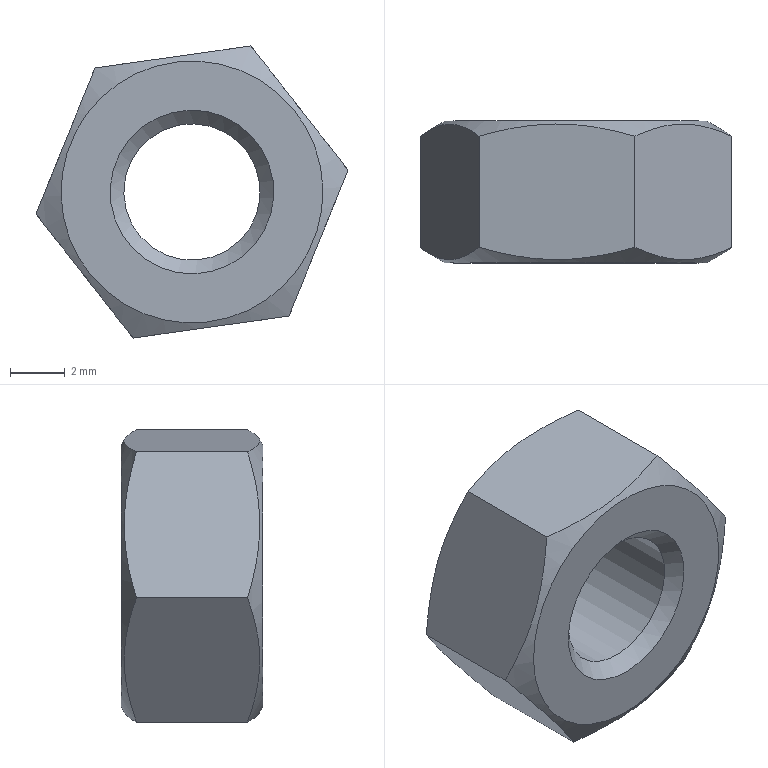Part | NX | features 倒角1 2 | 1 solid | 13 faces | box 11.434 x 5.2 x 10.707 mm | volume 339.24 mm3 | plane 8 | cone 4 | cylinder 1 | commonest cylinder face diameters 5 x1
STEP:
#1=CARTESIAN_POINT('',(16.564,347.416,103.063));
#2=VERTEX_POINT('',#1);
#3=CARTESIAN_POINT('',(17.5,347.416,105.381));
#4=DIRECTION('',(0.,1.,0.));
#5=DIRECTION('',(-0.3744,0.,-0.9273));
#6=AXIS2_PLACEMENT_3D('',#3,#4,#5);
#7=CIRCLE('',#6,2.5);
#8=EDGE_CURVE('',#2,#2,#7,.T.);
#9=ORIENTED_EDGE('',*,*,#8,.F.);
#10=EDGE_LOOP('',(#9));
#11=FACE_BOUND('',#10,.T.);
#12=CARTESIAN_POINT('',(16.377,347.916,102.599));
#13=VERTEX_POINT('',#12);
#14=CARTESIAN_POINT('',(17.5,347.916,105.381));
#15=DIRECTION('',(0.,-1.,0.));
#16=DIRECTION('',(-0.3744,0.,-0.9273));
#17=AXIS2_PLACEMENT_3D('',#14,#15,#16);
#18=CIRCLE('',#17,3.);
#19=EDGE_CURVE('',#13,#13,#18,.T.);
#20=ORIENTED_EDGE('',*,*,#19,.F.);
#21=EDGE_LOOP('',(#20));
#22=FACE_BOUND('',#21,.T.);
#23=CARTESIAN_POINT('',(17.5,347.416,105.381));
#24=DIRECTION('',(0.,1.,0.));
#25=DIRECTION('',(0.3744,0.,0.9273));
#26=AXIS2_PLACEMENT_3D('',#23,#24,#25);
#27=CONICAL_SURFACE('',#26,2.5,0.7854);
#28=ADVANCED_FACE('',(#11,#22),#27,.F.);
#29=CARTESIAN_POINT('',(16.377,342.716,102.599));
#30=VERTEX_POINT('',#29);
#31=CARTESIAN_POINT('',(17.5,342.716,105.381));
#32=DIRECTION('',(0.,1.,0.));
#33=DIRECTION('',(-0.3744,0.,-0.9273));
#34=AXIS2_PLACEMENT_3D('',#31,#32,#33);
#35=CIRCLE('',#34,3.);
#36=EDGE_CURVE('',#30,#30,#35,.T.);
#37=ORIENTED_EDGE('',*,*,#36,.F.);
#38=EDGE_LOOP('',(#37));
#39=FACE_BOUND('',#38,.T.);
#40=CARTESIAN_POINT('',(16.564,343.216,103.063));
#41=VERTEX_POINT('',#40);
#42=CARTESIAN_POINT('',(17.5,343.216,105.381));
#43=DIRECTION('',(0.,-1.,0.));
#44=DIRECTION('',(-0.3744,0.,-0.9273));
#45=AXIS2_PLACEMENT_3D('',#42,#43,#44);
#46=CIRCLE('',#45,2.5);
#47=EDGE_CURVE('',#41,#41,#46,.T.);
#48=ORIENTED_EDGE('',*,*,#47,.F.);
#49=EDGE_LOOP('',(#48));
#50=FACE_BOUND('',#49,.T.);
#51=CARTESIAN_POINT('',(17.5,342.716,105.381));
#52=DIRECTION('',(0.,-1.,0.));
#53=DIRECTION('',(-0.3744,0.,-0.9273));
#54=AXIS2_PLACEMENT_3D('',#51,#52,#53);
#55=CONICAL_SURFACE('',#54,3.,0.7854);
#56=ADVANCED_FACE('',(#39,#50),#55,.F.);
#57=CARTESIAN_POINT('',(13.945,347.354,109.93));
#58=VERTEX_POINT('',#57);
#59=CARTESIAN_POINT('',(19.662,347.354,110.735));
#60=VERTEX_POINT('',#59);
#61=CARTESIAN_POINT('',(13.945,347.354,109.93));
#62=CARTESIAN_POINT('',(14.878,347.626,110.061));
#63=CARTESIAN_POINT('',(16.793,347.975,110.331));
#64=CARTESIAN_POINT('',(18.727,347.626,110.603));
#65=CARTESIAN_POINT('',(19.662,347.354,110.735));
#66=B_SPLINE_CURVE_WITH_KNOTS('',3,(#61,#62,#63,#64,#65),.UNSPECIFIED.,.F.,.F.,(4,1,4),(0.,0.002915,0.005831),.UNSPECIFIED.);
#67=EDGE_CURVE('',#58,#60,#66,.T.);
#68=ORIENTED_EDGE('',*,*,#67,.T.);
#69=CARTESIAN_POINT('',(23.217,347.354,106.186));
#70=VERTEX_POINT('',#69);
#71=CARTESIAN_POINT('',(19.662,347.354,110.735));
#72=CARTESIAN_POINT('',(20.242,347.626,109.992));
#73=CARTESIAN_POINT('',(21.433,347.975,108.469));
#74=CARTESIAN_POINT('',(22.636,347.626,106.93));
#75=CARTESIAN_POINT('',(23.217,347.354,106.186));
#76=B_SPLINE_CURVE_WITH_KNOTS('',3,(#71,#72,#73,#74,#75),.UNSPECIFIED.,.F.,.F.,(4,1,4),(0.,0.002915,0.005831),.UNSPECIFIED.);
#77=EDGE_CURVE('',#60,#70,#76,.T.);
#78=ORIENTED_EDGE('',*,*,#77,.T.);
#79=CARTESIAN_POINT('',(21.055,347.354,100.832));
#80=VERTEX_POINT('',#79);
#81=CARTESIAN_POINT('',(23.217,347.354,106.186));
#82=CARTESIAN_POINT('',(22.864,347.626,105.312));
#83=CARTESIAN_POINT('',(22.14,347.975,103.519));
#84=CARTESIAN_POINT('',(21.409,347.626,101.708));
#85=CARTESIAN_POINT('',(21.055,347.354,100.832));
#86=B_SPLINE_CURVE_WITH_KNOTS('',3,(#81,#82,#83,#84,#85),.UNSPECIFIED.,.F.,.F.,(4,1,4),(0.,0.002915,0.005831),.UNSPECIFIED.);
#87=EDGE_CURVE('',#70,#80,#86,.T.);
#88=ORIENTED_EDGE('',*,*,#87,.T.);
#89=CARTESIAN_POINT('',(15.338,347.354,100.028));
#90=VERTEX_POINT('',#89);
#91=CARTESIAN_POINT('',(21.055,347.354,100.832));
#92=CARTESIAN_POINT('',(20.122,347.626,100.701));
#93=CARTESIAN_POINT('',(18.207,347.975,100.431));
#94=CARTESIAN_POINT('',(16.273,347.626,100.159));
#95=CARTESIAN_POINT('',(15.338,347.354,100.028));
#96=B_SPLINE_CURVE_WITH_KNOTS('',3,(#91,#92,#93,#94,#95),.UNSPECIFIED.,.F.,.F.,(4,1,4),(0.,0.002915,0.005831),.UNSPECIFIED.);
#97=EDGE_CURVE('',#80,#90,#96,.T.);
#98=ORIENTED_EDGE('',*,*,#97,.T.);
#99=CARTESIAN_POINT('',(11.783,347.354,104.576));
#100=VERTEX_POINT('',#99);
#101=CARTESIAN_POINT('',(15.338,347.354,100.028));
#102=CARTESIAN_POINT('',(14.758,347.626,100.77));
#103=CARTESIAN_POINT('',(13.567,347.975,102.294));
#104=CARTESIAN_POINT('',(12.364,347.626,103.833));
#105=CARTESIAN_POINT('',(11.783,347.354,104.576));
#106=B_SPLINE_CURVE_WITH_KNOTS('',3,(#101,#102,#103,#104,#105),.UNSPECIFIED.,.F.,.F.,(4,1,4),(0.,0.002915,0.005831),.UNSPECIFIED.);
#107=EDGE_CURVE('',#90,#100,#106,.T.);
#108=ORIENTED_EDGE('',*,*,#107,.T.);
#109=CARTESIAN_POINT('',(11.783,347.354,104.576));
#110=CARTESIAN_POINT('',(12.136,347.626,105.451));
#111=CARTESIAN_POINT('',(12.86,347.975,107.244));
#112=CARTESIAN_POINT('',(13.591,347.626,109.055));
#113=CARTESIAN_POINT('',(13.945,347.354,109.93));
#114=B_SPLINE_CURVE_WITH_KNOTS('',3,(#109,#110,#111,#112,#113),.UNSPECIFIED.,.F.,.F.,(4,1,4),(0.,0.002915,0.005831),.UNSPECIFIED.);
#115=EDGE_CURVE('',#100,#58,#114,.T.);
#116=ORIENTED_EDGE('',*,*,#115,.T.);
#117=EDGE_LOOP('',(#68,#78,#88,#98,#108,#116));
#118=FACE_BOUND('',#117,.T.);
#119=CARTESIAN_POINT('',(19.297,347.916,109.832));
#120=VERTEX_POINT('',#119);
#121=CARTESIAN_POINT('',(17.5,347.916,105.381));
#122=DIRECTION('',(0.,-1.,0.));
#123=DIRECTION('',(0.3744,0.,0.9273));
#124=AXIS2_PLACEMENT_3D('',#121,#122,#123);
#125=CIRCLE('',#124,4.8);
#126=EDGE_CURVE('',#120,#120,#125,.T.);
#127=ORIENTED_EDGE('',*,*,#126,.T.);
#128=EDGE_LOOP('',(#127));
#129=FACE_BOUND('',#128,.T.);
#130=CARTESIAN_POINT('',(17.5,347.354,105.381));
#131=DIRECTION('',(0.,-1.,0.));
#132=DIRECTION('',(-0.3744,0.,-0.9273));
#133=AXIS2_PLACEMENT_3D('',#130,#131,#132);
#134=CONICAL_SURFACE('',#133,5.774,1.047);
#135=ADVANCED_FACE('',(#118,#129),#134,.T.);
#136=CARTESIAN_POINT('',(19.297,342.716,109.832));
#137=VERTEX_POINT('',#136);
#138=CARTESIAN_POINT('',(17.5,342.716,105.381));
#139=DIRECTION('',(0.,-1.,0.));
#140=DIRECTION('',(0.3744,0.,0.9273));
#141=AXIS2_PLACEMENT_3D('',#138,#139,#140);
#142=CIRCLE('',#141,4.8);
#143=EDGE_CURVE('',#137,#137,#142,.T.);
#144=ORIENTED_EDGE('',*,*,#143,.F.);
#145=EDGE_LOOP('',(#144));
#146=FACE_BOUND('',#145,.T.);
#147=CARTESIAN_POINT('',(11.783,343.278,104.576));
#148=VERTEX_POINT('',#147);
#149=CARTESIAN_POINT('',(15.338,343.278,100.028));
#150=VERTEX_POINT('',#149);
#151=CARTESIAN_POINT('',(11.783,343.278,104.576));
#152=CARTESIAN_POINT('',(12.363,343.006,103.834));
#153=CARTESIAN_POINT('',(13.554,342.657,102.31));
#154=CARTESIAN_POINT('',(14.757,343.005,100.771));
#155=CARTESIAN_POINT('',(15.338,343.278,100.028));
#156=B_SPLINE_CURVE_WITH_KNOTS('',3,(#151,#152,#153,#154,#155),.UNSPECIFIED.,.F.,.F.,(4,1,4),(0.,0.002915,0.005831),.UNSPECIFIED.);
#157=EDGE_CURVE('',#148,#150,#156,.T.);
#158=ORIENTED_EDGE('',*,*,#157,.T.);
#159=CARTESIAN_POINT('',(21.055,343.278,100.832));
#160=VERTEX_POINT('',#159);
#161=CARTESIAN_POINT('',(15.338,343.278,100.028));
#162=CARTESIAN_POINT('',(16.272,343.006,100.159));
#163=CARTESIAN_POINT('',(18.187,342.657,100.429));
#164=CARTESIAN_POINT('',(20.121,343.005,100.701));
#165=CARTESIAN_POINT('',(21.055,343.278,100.832));
#166=B_SPLINE_CURVE_WITH_KNOTS('',3,(#161,#162,#163,#164,#165),.UNSPECIFIED.,.F.,.F.,(4,1,4),(0.,0.002915,0.005831),.UNSPECIFIED.);
#167=EDGE_CURVE('',#150,#160,#166,.T.);
#168=ORIENTED_EDGE('',*,*,#167,.T.);
#169=CARTESIAN_POINT('',(23.217,343.278,106.186));
#170=VERTEX_POINT('',#169);
#171=CARTESIAN_POINT('',(21.055,343.278,100.832));
#172=CARTESIAN_POINT('',(21.408,343.006,101.707));
#173=CARTESIAN_POINT('',(22.132,342.657,103.499));
#174=CARTESIAN_POINT('',(22.864,343.005,105.311));
#175=CARTESIAN_POINT('',(23.217,343.278,106.186));
#176=B_SPLINE_CURVE_WITH_KNOTS('',3,(#171,#172,#173,#174,#175),.UNSPECIFIED.,.F.,.F.,(4,1,4),(0.,0.002915,0.005831),.UNSPECIFIED.);
#177=EDGE_CURVE('',#160,#170,#176,.T.);
#178=ORIENTED_EDGE('',*,*,#177,.T.);
#179=CARTESIAN_POINT('',(19.662,343.278,110.735));
#180=VERTEX_POINT('',#179);
#181=CARTESIAN_POINT('',(23.217,343.278,106.186));
#182=CARTESIAN_POINT('',(22.637,343.006,106.929));
#183=CARTESIAN_POINT('',(21.446,342.657,108.452));
#184=CARTESIAN_POINT('',(20.243,343.005,109.991));
#185=CARTESIAN_POINT('',(19.662,343.278,110.735));
#186=B_SPLINE_CURVE_WITH_KNOTS('',3,(#181,#182,#183,#184,#185),.UNSPECIFIED.,.F.,.F.,(4,1,4),(0.,0.002915,0.005831),.UNSPECIFIED.);
#187=EDGE_CURVE('',#170,#180,#186,.T.);
#188=ORIENTED_EDGE('',*,*,#187,.T.);
#189=CARTESIAN_POINT('',(13.945,343.278,109.93));
#190=VERTEX_POINT('',#189);
#191=CARTESIAN_POINT('',(19.662,343.278,110.735));
#192=CARTESIAN_POINT('',(18.728,343.006,110.603));
#193=CARTESIAN_POINT('',(16.813,342.657,110.334));
#194=CARTESIAN_POINT('',(14.879,343.005,110.062));
#195=CARTESIAN_POINT('',(13.945,343.278,109.93));
#196=B_SPLINE_CURVE_WITH_KNOTS('',3,(#191,#192,#193,#194,#195),.UNSPECIFIED.,.F.,.F.,(4,1,4),(0.,0.002915,0.005831),.UNSPECIFIED.);
#197=EDGE_CURVE('',#180,#190,#196,.T.);
#198=ORIENTED_EDGE('',*,*,#197,.T.);
#199=CARTESIAN_POINT('',(13.945,343.278,109.93));
#200=CARTESIAN_POINT('',(13.592,343.006,109.056));
#201=CARTESIAN_POINT('',(12.868,342.657,107.263));
#202=CARTESIAN_POINT('',(12.136,343.005,105.452));
#203=CARTESIAN_POINT('',(11.783,343.278,104.576));
#204=B_SPLINE_CURVE_WITH_KNOTS('',3,(#199,#200,#201,#202,#203),.UNSPECIFIED.,.F.,.F.,(4,1,4),(0.,0.002915,0.005831),.UNSPECIFIED.);
#205=EDGE_CURVE('',#190,#148,#204,.T.);
#206=ORIENTED_EDGE('',*,*,#205,.T.);
#207=EDGE_LOOP('',(#158,#168,#178,#188,#198,#206));
#208=FACE_BOUND('',#207,.T.);
#209=CARTESIAN_POINT('',(17.5,342.716,105.381));
#210=DIRECTION('',(0.,1.,0.));
#211=DIRECTION('',(0.3744,0.,0.9273));
#212=AXIS2_PLACEMENT_3D('',#209,#210,#211);
#213=CONICAL_SURFACE('',#212,4.8,1.047);
#214=ADVANCED_FACE('',(#146,#208),#213,.T.);
#215=ORIENTED_EDGE('',*,*,#47,.T.);
#216=EDGE_LOOP('',(#215));
#217=FACE_BOUND('',#216,.T.);
#218=ORIENTED_EDGE('',*,*,#8,.T.);
#219=EDGE_LOOP('',(#218));
#220=FACE_BOUND('',#219,.T.);
#221=CARTESIAN_POINT('',(17.5,347.916,105.381));
#222=DIRECTION('',(0.,-1.,0.));
#223=DIRECTION('',(-0.3744,0.,-0.9273));
#224=AXIS2_PLACEMENT_3D('',#221,#222,#223);
#225=CYLINDRICAL_SURFACE('',#224,2.5);
#226=ADVANCED_FACE('',(#217,#220),#225,.F.);
#227=ORIENTED_EDGE('',*,*,#97,.F.);
#228=CARTESIAN_POINT('',(21.055,347.916,100.832));
#229=DIRECTION('',(0.,-1.,0.));
#230=VECTOR('',#229,1000.);
#231=LINE('',#228,#230);
#232=EDGE_CURVE('',#80,#160,#231,.T.);
#233=ORIENTED_EDGE('',*,*,#232,.T.);
#234=ORIENTED_EDGE('',*,*,#167,.F.);
#235=CARTESIAN_POINT('',(15.338,347.916,100.028));
#236=DIRECTION('',(0.,-1.,0.));
#237=VECTOR('',#236,1000.);
#238=LINE('',#235,#237);
#239=EDGE_CURVE('',#90,#150,#238,.T.);
#240=ORIENTED_EDGE('',*,*,#239,.F.);
#241=EDGE_LOOP('',(#227,#233,#234,#240));
#242=FACE_BOUND('',#241,.T.);
#243=CARTESIAN_POINT('',(21.055,347.916,100.832));
#244=DIRECTION('',(-0.1394,0.,0.9902));
#245=DIRECTION('',(-0.9902,0.,-0.1394));
#246=AXIS2_PLACEMENT_3D('',#243,#244,#245);
#247=PLANE('',#246);
#248=ADVANCED_FACE('',(#242),#247,.F.);
#249=ORIENTED_EDGE('',*,*,#107,.F.);
#250=ORIENTED_EDGE('',*,*,#239,.T.);
#251=ORIENTED_EDGE('',*,*,#157,.F.);
#252=CARTESIAN_POINT('',(11.783,347.916,104.576));
#253=DIRECTION('',(0.,-1.,0.));
#254=VECTOR('',#253,1000.);
#255=LINE('',#252,#254);
#256=EDGE_CURVE('',#100,#148,#255,.T.);
#257=ORIENTED_EDGE('',*,*,#256,.F.);
#258=EDGE_LOOP('',(#249,#250,#251,#257));
#259=FACE_BOUND('',#258,.T.);
#260=CARTESIAN_POINT('',(15.338,347.916,100.028));
#261=DIRECTION('',(0.7879,0.,0.6158));
#262=DIRECTION('',(-0.6158,0.,0.7879));
#263=AXIS2_PLACEMENT_3D('',#260,#261,#262);
#264=PLANE('',#263);
#265=ADVANCED_FACE('',(#259),#264,.F.);
#266=ORIENTED_EDGE('',*,*,#115,.F.);
#267=ORIENTED_EDGE('',*,*,#256,.T.);
#268=ORIENTED_EDGE('',*,*,#205,.F.);
#269=CARTESIAN_POINT('',(13.945,347.916,109.93));
#270=DIRECTION('',(0.,-1.,0.));
#271=VECTOR('',#270,1000.);
#272=LINE('',#269,#271);
#273=EDGE_CURVE('',#58,#190,#272,.T.);
#274=ORIENTED_EDGE('',*,*,#273,.F.);
#275=EDGE_LOOP('',(#266,#267,#268,#274));
#276=FACE_BOUND('',#275,.T.);
#277=CARTESIAN_POINT('',(11.783,347.916,104.576));
#278=DIRECTION('',(0.9273,0.,-0.3744));
#279=DIRECTION('',(0.,1.,0.));
#280=AXIS2_PLACEMENT_3D('',#277,#278,#279);
#281=PLANE('',#280);
#282=ADVANCED_FACE('',(#276),#281,.F.);
#283=ORIENTED_EDGE('',*,*,#67,.F.);
#284=ORIENTED_EDGE('',*,*,#273,.T.);
#285=ORIENTED_EDGE('',*,*,#197,.F.);
#286=CARTESIAN_POINT('',(19.662,347.916,110.735));
#287=DIRECTION('',(0.,-1.,0.));
#288=VECTOR('',#287,1000.);
#289=LINE('',#286,#288);
#290=EDGE_CURVE('',#60,#180,#289,.T.);
#291=ORIENTED_EDGE('',*,*,#290,.F.);
#292=EDGE_LOOP('',(#283,#284,#285,#291));
#293=FACE_BOUND('',#292,.T.);
#294=CARTESIAN_POINT('',(13.945,347.916,109.93));
#295=DIRECTION('',(0.1394,0.,-0.9902));
#296=DIRECTION('',(0.9902,0.,0.1394));
#297=AXIS2_PLACEMENT_3D('',#294,#295,#296);
#298=PLANE('',#297);
#299=ADVANCED_FACE('',(#293),#298,.F.);
#300=ORIENTED_EDGE('',*,*,#77,.F.);
#301=ORIENTED_EDGE('',*,*,#290,.T.);
#302=ORIENTED_EDGE('',*,*,#187,.F.);
#303=CARTESIAN_POINT('',(23.217,347.916,106.186));
#304=DIRECTION('',(0.,-1.,0.));
#305=VECTOR('',#304,1000.);
#306=LINE('',#303,#305);
#307=EDGE_CURVE('',#70,#170,#306,.T.);
#308=ORIENTED_EDGE('',*,*,#307,.F.);
#309=EDGE_LOOP('',(#300,#301,#302,#308));
#310=FACE_BOUND('',#309,.T.);
#311=CARTESIAN_POINT('',(19.662,347.916,110.735));
#312=DIRECTION('',(-0.7879,0.,-0.6158));
#313=DIRECTION('',(0.6158,0.,-0.7879));
#314=AXIS2_PLACEMENT_3D('',#311,#312,#313);
#315=PLANE('',#314);
#316=ADVANCED_FACE('',(#310),#315,.F.);
#317=ORIENTED_EDGE('',*,*,#87,.F.);
#318=ORIENTED_EDGE('',*,*,#307,.T.);
#319=ORIENTED_EDGE('',*,*,#177,.F.);
#320=ORIENTED_EDGE('',*,*,#232,.F.);
#321=EDGE_LOOP('',(#317,#318,#319,#320));
#322=FACE_BOUND('',#321,.T.);
#323=CARTESIAN_POINT('',(23.217,347.916,106.186));
#324=DIRECTION('',(-0.9273,0.,0.3744));
#325=DIRECTION('',(0.,-1.,0.));
#326=AXIS2_PLACEMENT_3D('',#323,#324,#325);
#327=PLANE('',#326);
#328=ADVANCED_FACE('',(#322),#327,.F.);
#329=ORIENTED_EDGE('',*,*,#19,.T.);
#330=EDGE_LOOP('',(#329));
#331=FACE_BOUND('',#330,.T.);
#332=ORIENTED_EDGE('',*,*,#126,.F.);
#333=EDGE_LOOP('',(#332));
#334=FACE_BOUND('',#333,.T.);
#335=CARTESIAN_POINT('',(17.5,347.916,105.381));
#336=DIRECTION('',(0.,1.,0.));
#337=DIRECTION('',(0.3744,0.,0.9273));
#338=AXIS2_PLACEMENT_3D('',#335,#336,#337);
#339=PLANE('',#338);
#340=ADVANCED_FACE('',(#331,#334),#339,.T.);
#341=ORIENTED_EDGE('',*,*,#36,.T.);
#342=EDGE_LOOP('',(#341));
#343=FACE_BOUND('',#342,.T.);
#344=ORIENTED_EDGE('',*,*,#143,.T.);
#345=EDGE_LOOP('',(#344));
#346=FACE_BOUND('',#345,.T.);
#347=CARTESIAN_POINT('',(17.5,342.716,105.381));
#348=DIRECTION('',(0.,1.,0.));
#349=DIRECTION('',(0.3744,0.,0.9273));
#350=AXIS2_PLACEMENT_3D('',#347,#348,#349);
#351=PLANE('',#350);
#352=ADVANCED_FACE('',(#343,#346),#351,.F.);
#353=CLOSED_SHELL('',(#28,#56,#135,#214,#226,#248,#265,#282,#299,#316,#328,#340,#352));
#354=MANIFOLD_SOLID_BREP('',#353);
#355=(LENGTH_UNIT()NAMED_UNIT(*)SI_UNIT(.MILLI.,.METRE.));
#356=UNCERTAINTY_MEASURE_WITH_UNIT(LENGTH_MEASURE(0.0508),#355,'','');
#357=(NAMED_UNIT(*)PLANE_ANGLE_UNIT()SI_UNIT($,.RADIAN.));
#358=(NAMED_UNIT(*)SI_UNIT($,.STERADIAN.)SOLID_ANGLE_UNIT());
#359=(GEOMETRIC_REPRESENTATION_CONTEXT(3)GLOBAL_UNCERTAINTY_ASSIGNED_CONTEXT((#356))GLOBAL_UNIT_ASSIGNED_CONTEXT((#355,#357,#358))REPRESENTATION_CONTEXT('',''));
#360=ADVANCED_BREP_SHAPE_REPRESENTATION('',(#354),#359);